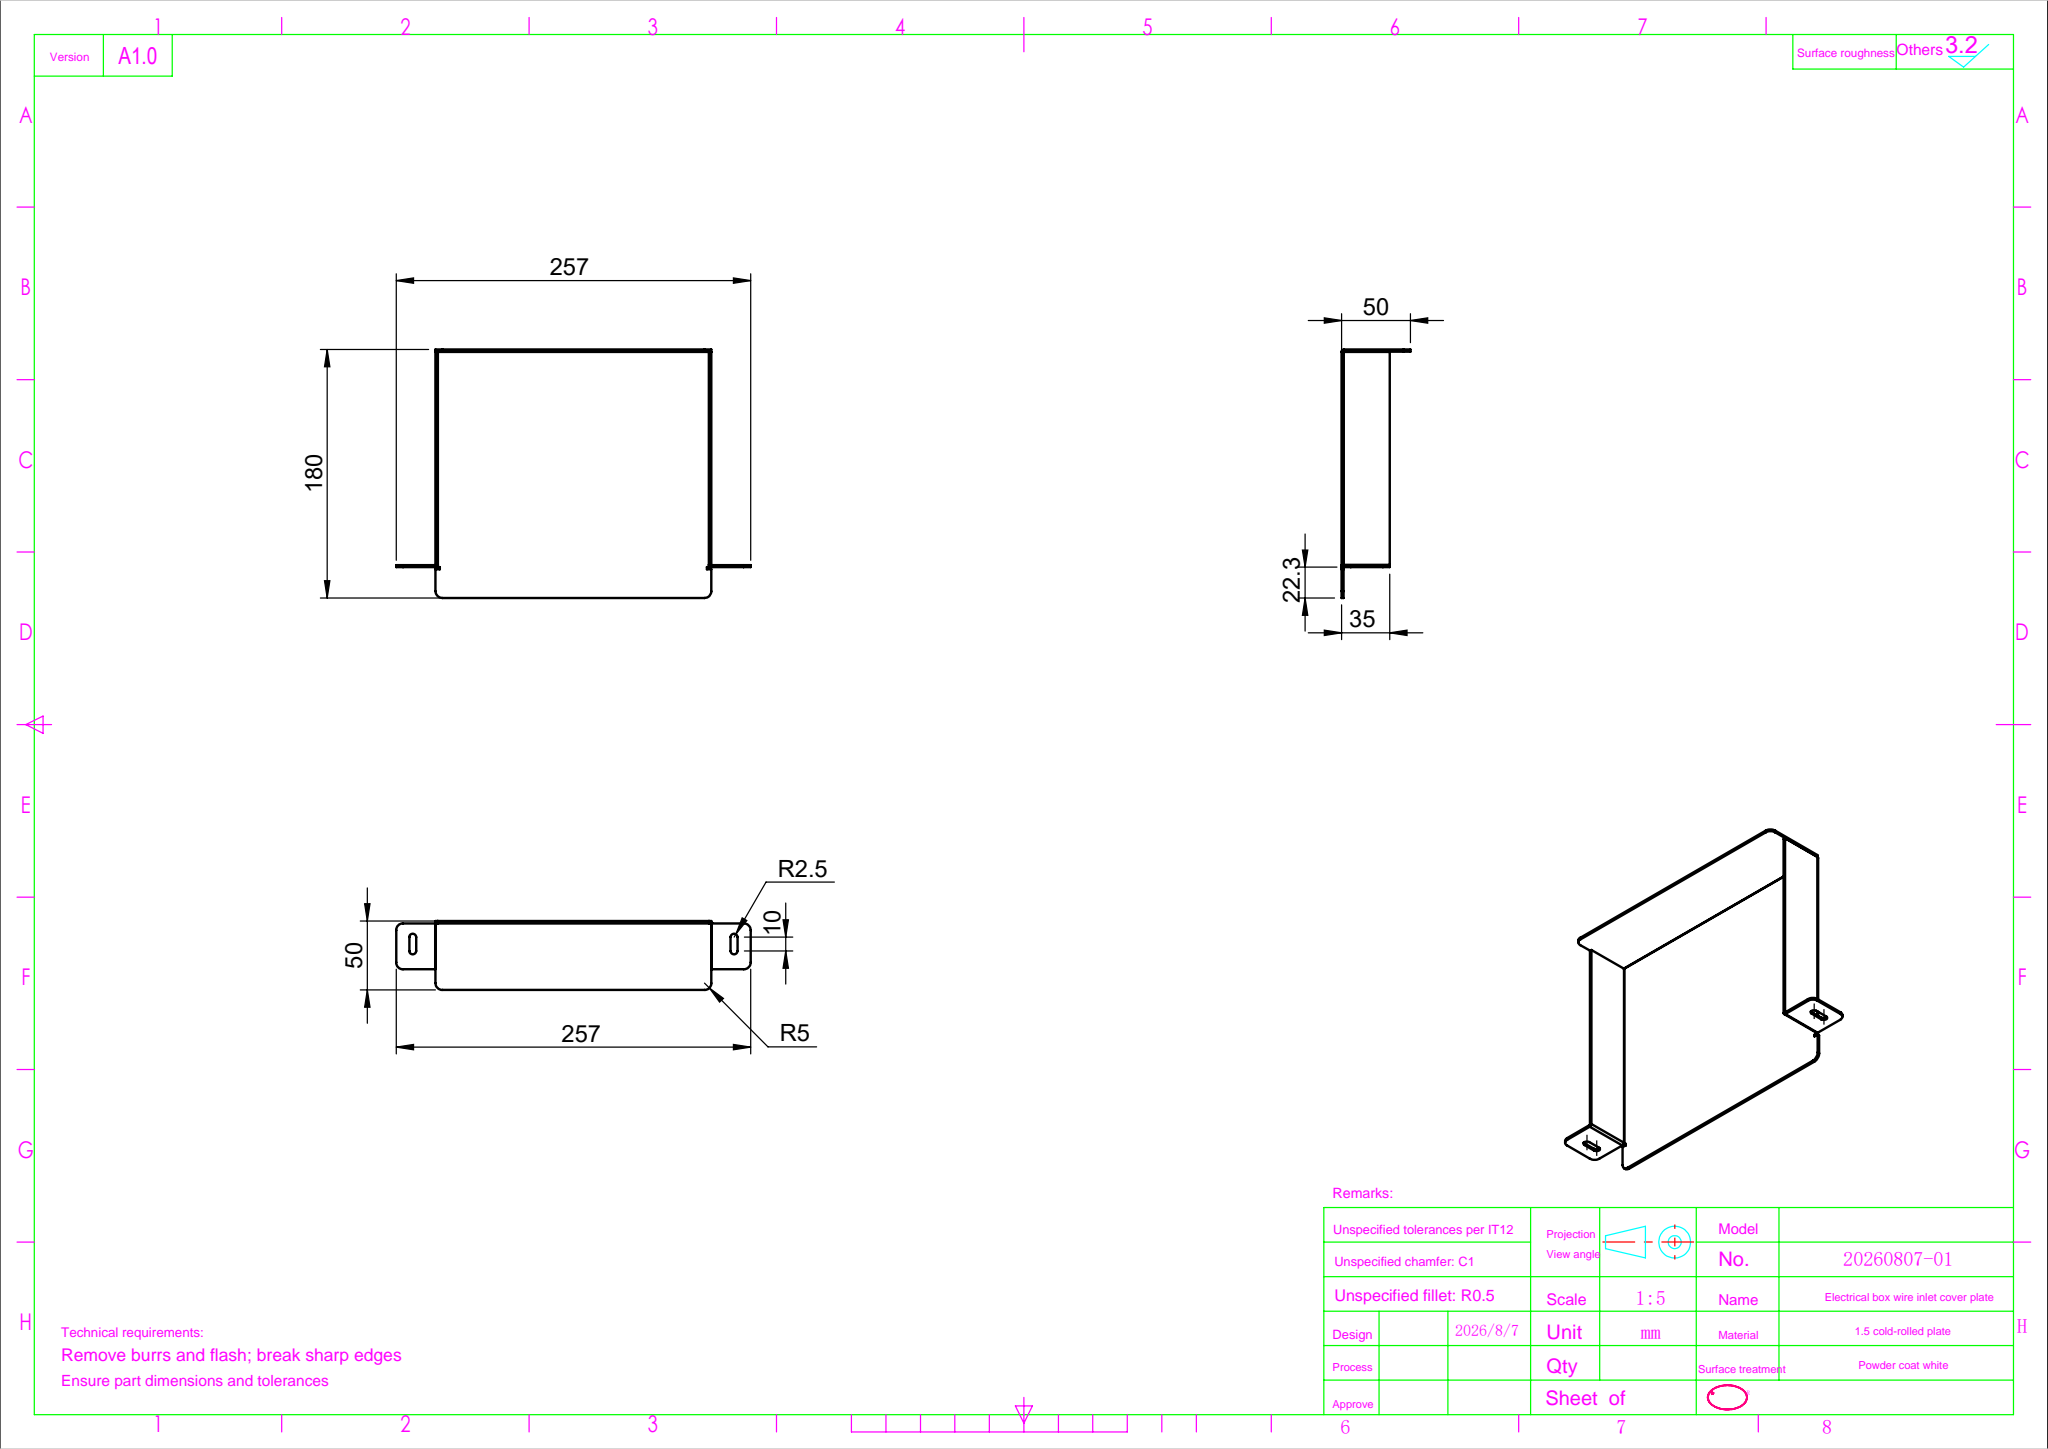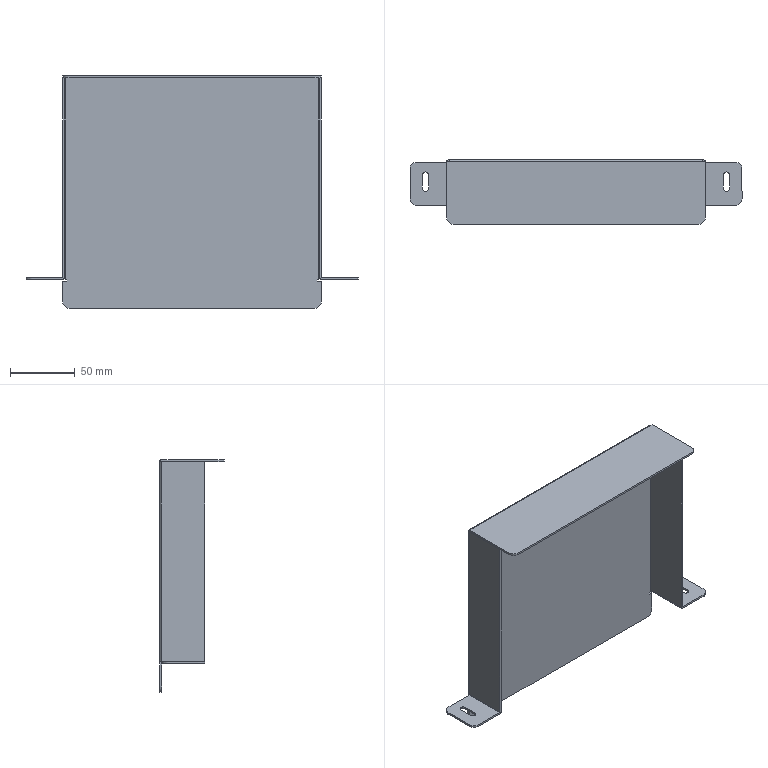Part | SolidWorks | features EdgeFlange 3, Fillet 3, FlatPattern 1, ICE 1, SMBaseFlange 1, SheetMetal 1 | 1 solid | 74 faces | box 257 x 50 x 180 mm | volume 86418 mm3 | plane 52 | cylinder 22 | commonest cylinder face diameters 10 x8 0.4 x5 3.4 x5 5 x4